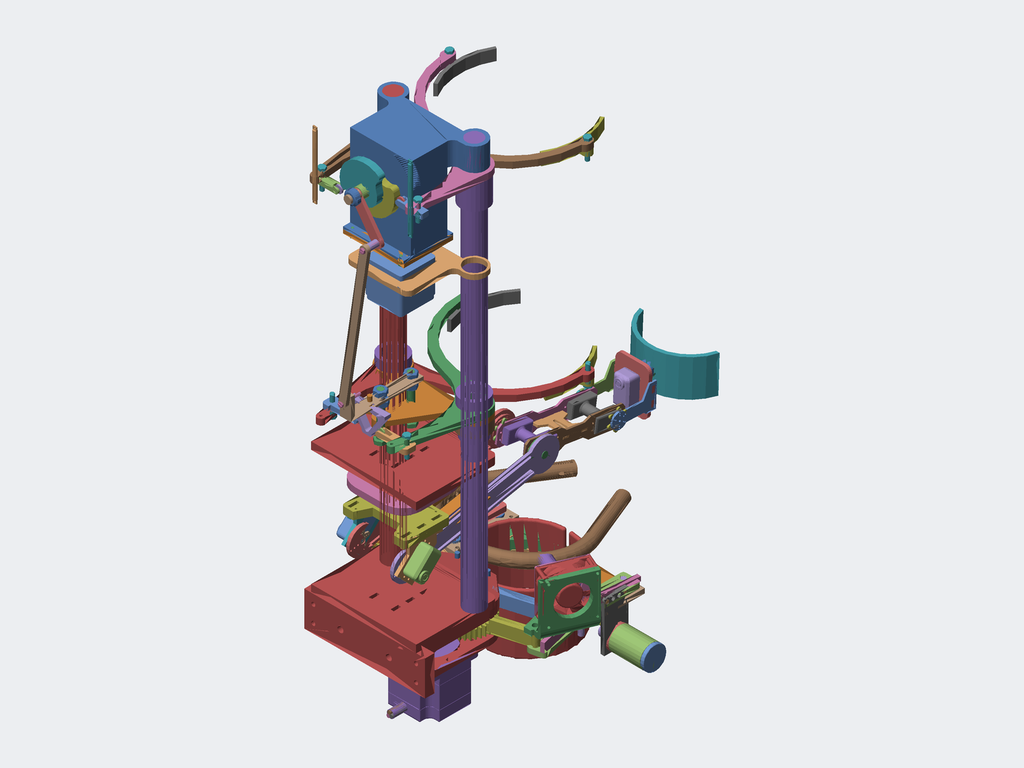Assembly | SolidWorks | 153 different items | 184 placed
Parts list (item | name | quantity | size | volume | features):
1 | (subassembly) | x1 | 346.952 x 128.874 x 340.963 mm | 1244535 mm3 | -
2 | - | x2 | 48 x 48 x 18 mm | 12158 mm3 | features Extrusion 1
3 | - | x1 | 42.805 x 27 x 33.95 mm | 11771 mm3 | features BaseBody 1
4 | - | x1 | 73.253 x 17.318 x 324 mm | 124814 mm3 | features BaseBody 1
5 | - | x1 | 225.335 x 227.919 x 57.4 mm | 931418 mm3 | features Cut 5, HoleWzd 5, ICE 3, Extrusion 1, Fillet 1
6 | - | x1 | 53.735 x 9.545 x 80 mm | 17956 mm3 | features BaseBody 1
7 | - | x1 | 20 x 23 x 32 mm | 12308 mm3 | features BaseBody 1
8 | - | x1 | 60 x 84 x 72 mm | 236948 mm3 | features ICE 5, Fillet 2, Chamfer 1, Extrusion 1
9 | - | x1 | 172 x 114 x 8 mm | 50080 mm3 | features Extrusion 1
10 | - | x1 | 40 x 24 x 32 mm | 2333 mm3 | features BaseBody 1
11 | - | x1 | 45 x 65 x 20 mm | 41025 mm3 | features BaseBody 1
12 | - | x1 | 40.811 x 30 x 4 mm | 1334 mm3 | features BaseBody 1
13 | - | x1 | 216 x 275.5 x 10 mm | 64163 mm3 | features Extrusion 1
14 | - | x1 | 200 x 37.759 x 140 mm | 122488 mm3 | features BaseBody 1
15 | - | x1 | 75.848 x 62.021 x 10 mm | 29978 mm3 | features Extrusion 1, ICE 1
16 | - | x1 | 75.848 x 62.021 x 10 mm | 30038 mm3 | features Extrusion 1, ICE 1
17 | - | x1 | 19.1 x 9.5 x 9.534 mm | 562.61 mm3 | features Extrusion 1, Fillet 1, ICE 1
18 | - | x1 | 19.1 x 9.5 x 9.534 mm | 562.61 mm3 | features Extrusion 1, Fillet 1, ICE 1
19 | - | x1 | 60 x 40 x 10 mm | 8175 mm3 | features Extrusion 1, ICE 1
20 | - | x1 | 23 x 23 x 4.6 mm | 774.952 mm3 | features Extrusion 1, ICE 1
21 | - | x1 | 39.607 x 26.395 x 3 mm | 406.832 mm3 | features BaseBody 1
22 | - | x1 | 31 x 75 x 3 mm | 697.725 mm3 | features BaseBody 1
23 | - | x1 | 102.526 x 43 x 3 mm | 1128 mm3 | features BaseBody 1
24 | - | x1 | 216 x 259.5 x 10 mm | 61129 mm3 | features Extrusion 1
25 | - | x1 | 30 x 13 x 10 mm | 1236 mm3 | features BaseBody 1
26 | - | x1 | 24.142 x 77.176 x 18 mm | 8760 mm3 | features BaseBody 1
27 | - | x1 | 20 x 20 x 20 mm | 5278 mm3 | features Extrusion 1
28 | - | x1 | 14.483 x 32 x 22.5 mm | 7805 mm3 | features BaseBody 1
29 | - | x1 | 28.933 x 49.206 x 26 mm | 4873 mm3 | features BaseBody 1
30 | - | x1 | 19.494 x 47.938 x 13 mm | 3166 mm3 | features BaseBody 1
31 | - | x1 | 29 x 12 x 12 mm | 1793 mm3 | features BaseBody 1
32 | - | x1 | 25.14 x 25.14 x 72 mm | 10941 mm3 | features BaseBody 1
33 | - | x1 | 8 x 14 x 80 mm | 2633 mm3 | features BaseBody 1
34 | - | x1 | 20 x 40 x 41 mm | 9841 mm3 | features BaseBody 1
35 | - | x1 | 44 x 12 x 8 mm | 3492 mm3 | features Extrusion 1, Fillet 1, ICE 1
36 | - | x1 | 42 x 13 x 13 mm | 2716 mm3 | features Chamfer 2, ICE 2, Revolution 1
37 | - | x1 | 114 x 17 x 17 mm | 14497 mm3 | features ICE 2, Revolution 1
38 | - | x1 | 18 x 18 x 10 mm | 1338 mm3 | features Extrusion 1
39 | - | x1 | 120 x 18 x 36 mm | 15012 mm3 | features ICE 5, Extrusion 1
40 | - | x1 | 12 x 106 x 27.4 mm | 23043 mm3 | features ICE 2, Extrusion 1, Fillet 1
41 | - | x1 | 12 x 106 x 27.4 mm | 23043 mm3 | features ICE 2, Extrusion 1, Fillet 1
42 | - | x1 | 77.185 x 16 x 5 mm | 5210 mm3 | features Extrusion 1
43 | - | x1 | 10 x 10 x 15.5 mm | 1023 mm3 | features Extrusion 1
44 | - | x1 | 252 x 12 x 6 mm | 17808 mm3 | features Extrusion 1
45 | - | x1 | 222.738 x 50.026 x 174 mm | 466487 mm3 | features BaseBody 1
46 | - | x1 | 44 x 12 x 8 mm | 3492 mm3 | features Extrusion 1, Fillet 1, ICE 1
47 | - | x1 | 60 x 84 x 72 mm | 237017 mm3 | features ICE 4, Fillet 2, Chamfer 1, Extrusion 1
48 | - | x1 | 216 x 263.5 x 15 mm | 92831 mm3 | features Extrusion 1
49 | - | x1 | 216 x 259.5 x 15 mm | 91694 mm3 | features Extrusion 1
50 | - | x1 | 2.5 x 53.856 x 24.571 mm | 1339 mm3 | features ICE 4, MoveCopyBody 1, Stock 1
51 | - | x1 | 2.5 x 53.856 x 24.571 mm | 1339 mm3 | features ICE 4, MoveCopyBody 1, Stock 1
52 | - | x1 | 90 x 15 x 10 mm | 13500 mm3 | features BaseBody 1
53 | - | x1 | 23.5 x 40.616 x 37 mm | 6167 mm3 | features BaseBody 1
54 | - | x1 | 105.6 x 75 x 12 mm | 72869 mm3 | features Extrusion 1
55 | - | x1 | 70 x 36.517 x 5 mm | 8161 mm3 | features Fillet 3, Extrusion 1
56 | - | x1 | 70 x 36.517 x 5 mm | 8161 mm3 | features Fillet 3, Extrusion 1
57 | - | x1 | 75.329 x 67.7 x 5 mm | 9212 mm3 | features Extrusion 1
58 | - | x1 | 75.329 x 67.7 x 5 mm | 9212 mm3 | features Extrusion 1
59 | - | x1 | 42.5 x 72.6 x 3 mm | 4588 mm3 | features Extrusion 1
60 | - | x1 | 33.41 x 29.789 x 5.85 mm | 1360 mm3 | features ICE 4, Extrusion 1, Fillet 1
61 | - | x1 | 33.41 x 29.789 x 5.85 mm | 1360 mm3 | features ICE 4, Extrusion 1, Fillet 1
62 | - | x1 | 33.41 x 29.789 x 5.85 mm | 1360 mm3 | features ICE 4, Extrusion 1, Fillet 1
63 | - | x1 | 33.41 x 29.789 x 5.85 mm | 1360 mm3 | features ICE 4, Extrusion 1, Fillet 1
64 | - | x1 | 33.41 x 29.789 x 5.85 mm | 1360 mm3 | features ICE 4, Extrusion 1, Fillet 1
65 | - | x1 | 33.41 x 29.789 x 5.85 mm | 1360 mm3 | features ICE 4, Extrusion 1, Fillet 1
66 | - | x1 | 33.41 x 29.789 x 5.85 mm | 1360 mm3 | features ICE 4, Extrusion 1, Fillet 1
67 | - | x1 | 171 x 118.5 x 140 mm | 515598 mm3 | features ICE 7, RevCut 2, Extrusion 1
68 | - | x1 | 82 x 100 x 14 mm | 49472 mm3 | features ICE 5, Extrusion 1
69 | - | x1 | 45.38 x 20.336 x 45.38 mm | 6966 mm3 | features BaseBody 1
70 | - | x1 | 65.7 x 75 x 5 mm | 16997 mm3 | features Extrusion 1, Fillet 1, ICE 1
71 | - | x1 | 50 x 20 x 50 mm | 8321 mm3 | features BaseBody 1
72 | - | x1 | - | - | features ICE 2, CirPattern 1, Extrusion 1, Helix 1, RefAxis 1, SweepCut 1
73 | - | x1 | 279.515 x 6.264 x 50 mm | 42669 mm3 | features ICE 3, Extrusion 1
74 | - | x1 | 279.515 x 6.264 x 50 mm | 42669 mm3 | features ICE 3, Extrusion 1
75 | - | x1 | 79 x 77.9 x 5 mm | 23665 mm3 | features Extrusion 1, ICE 1
76 | - | x1 | 77.052 x 77.02 x 12.051 mm | 23159 mm3 | features RefAxis 2, Revolution 2, BlendCut 1, CirPattern 1, ICE 1
77 | - | x1 | 671 x 37 x 37 mm | 528385 mm3 | features Revolution 1
78 | - | x1 | 671 x 44 x 44 mm | 560064 mm3 | features Revolution 1
79 | - | x1 | 17.234 x 17.234 x 54 mm | 6790 mm3 | features ICE 6, Chamfer 1, CirPattern 1, Extrusion 1, Helix 1, RefAxis 1, SweepCut 1
80 | - | x1 | 164.86 x 31.5 x 3 mm | 8343 mm3 | features Extrusion 1
81 | - | x1 | 54 x 20 x 8 mm | 4696 mm3 | features Fillet 2, ICE 2, Extrusion 1
82 | - | x1 | 164.86 x 31.5 x 3 mm | 8343 mm3 | features Extrusion 1
83 | - | x1 | 50 x 49.3 x 3 mm | 5034 mm3 | features Extrusion 1
84 | - | x1 | 40 x 15 x 40 mm | 6357 mm3 | features ICE 5, Extrusion 1
85 | - | x1 | 40 x 13.2 x 40 mm | 4095 mm3 | features ICE 5, Extrusion 1
86 | - | x1 | 41.5 x 21.5 x 55 mm | 30038 mm3 | features ICE 6, Chamfer 1, Extrusion 1, Fillet 1
87 | - | x1 | 41.5 x 21.5 x 55 mm | 30038 mm3 | features ICE 6, Chamfer 1, Extrusion 1, Fillet 1
88 | - | x1 | 29.446 x 29.325 x 13.992 mm | 4731 mm3 | features RefAxis 2, BlendCut 1, CirPattern 1, Revolution 1
89 | - | x1 | 50.144 x 42.117 x 46.062 mm | 27040 mm3 | features ICE 3, Fillet 2, Chamfer 1, Cut 1, Extrusion 1
90 | - | x1 | 50.144 x 42.117 x 46.062 mm | 27040 mm3 | features ICE 3, Fillet 2, Chamfer 1, Cut 1, Extrusion 1
91 | - | x1 | 50.144 x 42.117 x 46.062 mm | 27040 mm3 | features ICE 3, Fillet 2, Chamfer 1, Cut 1, Extrusion 1
92 | - | x1 | 54 x 20 x 8 mm | 4696 mm3 | features Fillet 2, ICE 2, Extrusion 1
93 | - | x2 | 174 x 136 x 12 mm | 259651 mm3 | features Extrusion 1, Fillet 1
94 | - | x1 | 110 x 110 x 25 mm | 105460 mm3 | features Fillet 2, ICE 2, Extrusion 1
95 | - | x1 | 50 x 50 x 36 mm | 14585 mm3 | features ICE 4, Extrusion 1
96 | - | x2 | 80 x 139.91 x 27.4 mm | 82359 mm3 | features ICE 3, Extrusion 1, Fillet 1
97 | - | x1 | 27.226 x 27.226 x 15 mm | 4643 mm3 | features Extrusion 1
98 | - | x1 | 6 x 6 x 110 mm | 2900 mm3 | features ICE 4, Extrusion 1
99 | - | x1 | 6 x 6 x 110 mm | 2900 mm3 | features ICE 4, Extrusion 1
100 | - | x2 | 20 x 20 x 10 mm | 2867 mm3 | features HoleWzd 2, Cut 1, Extrusion 1
101 | - | x4 | 3 x 3 x 13 mm | 89.797 mm3 | features Chamfer 1, Extrusion 1
102 | - | x4 | 12 x 12 x 46 mm | 2501 mm3 | features ICE 3, Extrusion 1
103 | - | x1 | 216 x 275.5 x 10 mm | 60864 mm3 | features Extrusion 1
104 | - | x2 | 31.948 x 20.133 x 14.168 mm | 1802 mm3 | features Cut 7, ICE 5, Extrusion 1, HoleWzd 1
105 | - | x2 | 111.649 x 70.016 x 8 mm | 27509 mm3 | features HoleWzd 3, ICE 3, Cut 1, Extrusion 1
106 | - | x2 | 6 x 19 x 6.001 mm | 500.74 mm3 | features Cut 3, Extrusion 1, HoleWzd 1
107 | - | x4 | 20 x 20 x 11 mm | 1797 mm3 | features Chamfer 1, Extrusion 1, ICE 1
108 | - | x2 | 5 x 5 x 15 mm | 142.965 mm3 | features ICE 2, Cut 1, Extrusion 1
109 | - | x2 | 5 x 5 x 19.999 mm | 180.305 mm3 | features ICE 2, Cut 1, Extrusion 1
110 | - | x1 | 176.98 x 108.741 x 8 mm | 42748 mm3 | features Cut 1, Extrusion 1
111 | - | x1 | 176.98 x 108.741 x 8 mm | 42748 mm3 | features Cut 1, Extrusion 1
112 | - | x1 | 166.528 x 92.061 x 15 mm | 14282 mm3 | features HoleWzd 2, Cut 1, Extrusion 1
113 | - | x1 | 166.528 x 92.061 x 15 mm | 14282 mm3 | features Cut 2, Extrusion 1, HoleWzd 1
114 | - | x1 | 216 x 275.5 x 10 mm | 60864 mm3 | features Extrusion 1
115 | - | x4 | 6 x 6 x 12 mm | 334.841 mm3 | features Chamfer 2, Extrusion 1
116 | - | x1 | 39.504 x 80 x 6.135 mm | 17187 mm3 | features Cut 2, HoleWzd 2, Extrusion 1
117 | - | x1 | 39.504 x 80 x 6.135 mm | 17187 mm3 | features Cut 2, HoleWzd 2, Extrusion 1
118 | - | x1 | 114.513 x 126.581 x 23 mm | 34516 mm3 | features Cut 4, HoleWzd 2, Extrusion 1, ICE 1
119 | - | x1 | 84.083 x 77.703 x 6 mm | 11123 mm3 | features Extrusion 1, ICE 1
120 | - | x1 | 88.743 x 86.001 x 87 mm | 61033 mm3 | features Cut 2, ICE 2, RefAxis 2, EdgeFlange 1, FlatPattern 1, SMBaseFlange 1, SheetMetal 1
121 | - | x2 | 70 x 70 x 25 mm | 39371 mm3 | features ICE 10, Fillet 8, CirPattern 2, MirrorPattern 2, CombineBodies 1, Extrusion 1, Helix 1, RevCut 1, Sweep 1
122 | - | x1 | 86.705 x 77.475 x 87.001 mm | 59436 mm3 | features Cut 1, EdgeFlange 1, FlatPattern 1, ICE 1, SMBaseFlange 1, SheetMetal 1
123 | - | x2 | 238.083 x 103.353 x 20 mm | 30963 mm3 | features RevCut 2, CirPattern 1, Cut 1, RefAxis 1, Sweep 1
124 | - | x2 | 50 x 50 x 56.352 mm | 10137 mm3 | features ICE 2, Blend 1, Cut 1, Extrusion 1, RefAxis 1, RevCut 1, SweepCut 1
125 | - | x1 | 182 x 122.5 x 22 mm | 68800 mm3 | features Extrusion 1, ICE 1
126 | - | x2 | 70 x 70 x 2 mm | 5744 mm3 | features Cut 2, FlatPattern 1, SMBaseFlange 1, SheetMetal 1
127 | - | x4 | 14 x 14 x 65.4 mm | 3691 mm3 | features ICE 2, Cut 1, Extrusion 1
128 | - | x1 | 114.513 x 126.581 x 23 mm | 34944 mm3 | features Cut 5, ICE 5, RevCut 3, HoleWzd 2, Extrusion 1
129 | - | x1 | 84.083 x 77.703 x 6 mm | 11123 mm3 | features Extrusion 1, ICE 1
130 | - | x2 | 139.296 x 94.506 x 100 mm | 127694 mm3 | features ICE 2, Extrusion 1, Fillet 1
131 | - | x1 | 24.068 x 19.259 x 24 mm | 2234 mm3 | features ICE 5, Fillet 2, Chamfer 1, Extrusion 1
132 | - | x1 | 12 x 12 x 2 mm | 201.062 mm3 | features Extrusion 1
133 | - | x1 | 12 x 12 x 2 mm | 201.062 mm3 | features Extrusion 1
134 | - | x1 | 12 x 12 x 2 mm | 201.062 mm3 | features Extrusion 1
135 | - | x1 | 12 x 12 x 2 mm | 201.062 mm3 | features Extrusion 1
136 | - | x2 | 44 x 44 x 63 mm | 26578 mm3 | features Extrusion 1, ICE 1
137 | - | x1 | 51.978 x 130.553 x 60 mm | 56854 mm3 | features Extrusion 1, ICE 1
138 | - | x1 | 35.397 x 105 x 18 mm | 11366 mm3 | features Extrusion 1, ICE 1
139 | - | x1 | 35.397 x 105 x 18 mm | 11366 mm3 | features Extrusion 1, ICE 1
140 | - | x1 | 35.397 x 105 x 18 mm | 11366 mm3 | features Extrusion 1, ICE 1
141 | - | x1 | 35.397 x 105 x 18 mm | 11366 mm3 | features Extrusion 1, ICE 1
142 | - | x1 | 85 x 105 x 109 mm | 475306 mm3 | features ICE 14, Fillet 8, Chamfer 3, CirPattern 2, Extrusion 1, MirrorPattern 1
143 | - | x1 | 50 x 43 x 48 mm | 49165 mm3 | features BaseBody 1
144 | - | x1 | 15 x 43.5 x 27 mm | 2257 mm3 | features BaseBody 1
145 | - | x1 | 55 x 55 x 44 mm | 106147 mm3 | features BaseBody 1
146 | - | x2 | 38 x 42.771 x 84 mm | 72893 mm3 | features Chamfer 4, Revolution 4, ICE 3, MirrorPattern 1, RefAxis 1
147 | - | x1 | 42.5 x 72.6 x 3 mm | 4588 mm3 | features Extrusion 1
148 | cross recessed hex bolts indentation gb | x1 | - | - | -
149 | hex bolts split pin hole-fine pitch-ab gb | x1 | - | - | -
150 | hex bolts with slot on head grade ab gb | x1 | - | - | -
151 | hex bolts with split pin hole-grade ab gb | x1 | - | - | -
152 | hex nuts 1-fine pitch-grades ab gb | x1 | - | - | -
153 | round nuts gb | x1 | - | - | -
Mates (type | each side: item.copy, entity, surface, feature):
Concentric | 67.1 face cylinder Boss-Extrude 1 | 78.1 face cylinder Revolve 1 | 2 times
Coincident | 67.1 edge | 78.1 edge
Concentric | 67.1 face cylinder Boss-Extrude 1 | 77.1 face cylinder Revolve 1
Coincident | 67.1 edge | 77.1 edge
Concentric | 77.1 face cylinder Revolve 1 | 13.1 face cylinder Boss-Extrude 1
Coincident | 77.1 face plane Revolve 1 | 13.1 face plane Boss-Extrude 1
Concentric | 78.1 face cylinder Revolve 1 | 24.1 face cylinder Boss-Extrude 1
Coincident | 78.1 face plane Revolve 1 | 24.1 face plane Boss-Extrude 1
Concentric | 24.1 face cylinder Boss-Extrude 1 | 140.1 face cylinder Boss-Extrude 5
Coincident | 24.1 face plane Boss-Extrude 1 | 140.1 face plane Boss-Extrude 5
Concentric | 13.1 face cylinder Boss-Extrude 1 | 141.1 face cylinder Boss-Extrude 5
Coincident | 13.1 face plane Boss-Extrude 1 | 141.1 face plane Boss-Extrude 5
Concentric | 24.1 face cylinder Boss-Extrude 1 | 98.1 face cylinder Boss-Extrude 1
Concentric | 13.1 face cylinder Boss-Extrude 1 | 99.1 face cylinder Boss-Extrude 1
Concentric | 24.1 face cylinder Boss-Extrude 1 | 35.1 face cylinder Boss-Extrude 1
Coincident | 24.1 face plane Boss-Extrude 1 | 35.1 face plane Boss-Extrude 1
Concentric | 35.1 face cylinder Boss-Extrude 2 | 132.1 face cylinder Boss-Extrude 1
DistanceDim | 132.1 face plane Boss-Extrude 1 | 35.1 face plane Boss-Extrude 1
Concentric | 13.1 face cylinder Boss-Extrude 1 | 46.1 face cylinder Boss-Extrude 1
Coincident | 13.1 face plane Boss-Extrude 1 | 46.1 face plane Boss-Extrude 1
Concentric | 46.1 face cylinder Boss-Extrude 2 | 133.1 face cylinder Boss-Extrude 1
DistanceDim | 133.1 face plane Boss-Extrude 1 | 46.1 face plane Boss-Extrude 1
Concentric | 67.1 face cylinder Cut-Revolve 3 | 37.1 face cylinder Revolve 1
Concentric | 37.1 face cylinder Revolve 1 | 72.1 face cylinder Cut-Extrude 1
Coincident | 67.1 face plane Boss-Extrude 7 | 72.1 face plane 0.80000 模数 , 78.1710mm P.D.
Concentric | 67.1 face cylinder Cut-Revolve 4 | 79.1 face cylinder Boss-Extrude 2
Coincident | 67.1 face plane Boss-Extrude 7 | 79.1 face plane Boss-Extrude 3
Concentric | 79.1 face cylinder Boss-Extrude 2 | 76.1 face cylinder 1.5 模数    , 76.5000mm P.D.
Coincident | 67.1 face plane Boss-Extrude 7 | 76.1 face plane Hub-Revolve1
Concentric | 68.1 face cylinder Cut-Extrude 9 | 20.1 face cylinder Boss-Extrude 2
Coincident | 68.1 face plane Boss-Extrude 3 | 20.1 edge
Concentric | 20.1 face cylinder Boss-Extrude 2 | 27.1 face cylinder Boss-Extrude 1
Coincident | 20.1 face plane Boss-Extrude 1 | 27.1 face plane Boss-Extrude 1
Concentric | 68.1 face cylinder Cut-Extrude 8 | 36.1 face cylinder Revolve 2
Coincident | 20.1 face plane Boss-Extrude 1 | 36.1 face plane Revolve 2
Concentric | 36.1 face cylinder Revolve 2 | 88.1 face cylinder 1.5 模数    , 25.5000mm P.D.
DistanceDim | 88.1 face plane 1.5 模数    , 25.5000mm P.D. | 36.1 face plane Revolve 2
Coincident | 67.1 face plane Boss-Extrude 1 | 37.1 face plane Revolve 1
Concentric | 37.1 face cylinder Revolve 1 | 15.1 face cylinder Boss-Extrude 1
Concentric | 37.1 face cylinder Revolve 1 | 16.1 face cylinder Boss-Extrude 1
ProfileCenter | 67.1 face plane Boss-Extrude 7 | 68.1 face plane Boss-Extrude 1
Concentric | 27.1 face cylinder Boss-Extrude 1 | 8.1 face cylinder Boss-Extrude 2
Coincident | 27.1 face plane Boss-Extrude 1 | 8.1 face plane Boss-Extrude 1
Concentric | 77.1 face cylinder Revolve 1 | 9.1 face cylinder Boss-Extrude 1
Concentric | 78.1 face cylinder Revolve 1 | 9.1 face cylinder Boss-Extrude 1
DistanceDim | 9.1 face plane Boss-Extrude 1 | 68.1 face plane Boss-Extrude 1
Parallel | 67.1 face plane Boss-Extrude 1 | 15.1 face plane Boss-Extrude 2 | 2 times
CamTangent | 15.1 face surface:4009 Boss-Extrude 2 | 132.1 face cylinder Boss-Extrude 1
Concentric | 37.1 face cylinder Revolve 1 | 38.1 face cylinder Boss-Extrude 1
Coincident | 16.1 face plane Boss-Extrude 2 | 38.1 face plane Boss-Extrude 1
Concentric | 37.1 face cylinder Revolve 1 | 42.1 face cylinder Boss-Extrude 1
Concentric | 42.1 face cylinder Boss-Extrude 1 | 43.1 face cylinder Boss-Extrude 1
Coincident | 42.1 face plane Boss-Extrude 1 | 43.1 face plane Boss-Extrude 1
Concentric | 43.1 face cylinder Boss-Extrude 1 | 44.1 face cylinder Boss-Extrude 1
Coincident | 43.1 face plane Boss-Extrude 1 | 44.1 face plane Boss-Extrude 1
Parallel | 37.1 face plane Cut-Extrude 1 | 38.1 face plane Boss-Extrude 1
Parallel | 38.1 face plane Boss-Extrude 1 | 42.1 face plane Boss-Extrude 1
Parallel | 37.1 face plane Cut-Extrude 1 | 15.1 face plane Boss-Extrude 2 | 2 times
Parallel | 37.1 face plane Cut-Extrude 1 | 16.1 face plane Boss-Extrude 2
Coincident | 15.1 face plane Boss-Extrude 2 | 16.1 face plane Boss-Extrude 2
CamTangent | 16.1 face surface:4009 Boss-Extrude 2 | 133.1 face cylinder Boss-Extrude 1
Concentric | 78.1 face cylinder Revolve 1 | 125.1 face cylinder Boss-Extrude 1
Concentric | 77.1 face cylinder Revolve 1 | 125.1 face cylinder Boss-Extrude 1
Parallel | 9.1 face plane Boss-Extrude 1 | 125.1 face plane Boss-Extrude 1
Concentric | 125.1 face cylinder Boss-Extrude 1 | 114.1 face cylinder Boss-Extrude 3
Coincident | 125.1 face plane Boss-Extrude 1 | 114.1 face plane Boss-Extrude 3
Concentric | 125.1 face cylinder Boss-Extrude 1 | 103.1 face cylinder Boss-Extrude 3
Coincident | 125.1 face plane Boss-Extrude 1 | 103.1 face plane Boss-Extrude 3
Concentric | 78.1 face cylinder Revolve 1 | 136.1 face cylinder Boss-Extrude 1
Coincident | 103.1 face plane Boss-Extrude 3 | 136.1 face plane Boss-Extrude 1
Coincident | 125.1 face plane Boss-Extrude 1 | 2.1 face plane Boss-Extrude 1
Concentric | 78.1 face cylinder Revolve 1 | 2.1 face cylinder Boss-Extrude 1
Concentric | 77.1 face cylinder Revolve 1 | 136.2 face cylinder Boss-Extrude 1
Coincident | 125.1 face plane Boss-Extrude 1 | 136.2 face plane Boss-Extrude 1
Concentric | 77.1 face cylinder Revolve 1 | 2.2 face cylinder Boss-Extrude 1
Coincident | 114.1 face plane Boss-Extrude 3 | 2.2 face plane Boss-Extrude 1
Concentric | 103.1 face cylinder Boss-Extrude 3 | 138.1 face cylinder Boss-Extrude 5
Coincident | 103.1 face plane Boss-Extrude 3 | 138.1 face plane Boss-Extrude 5
Concentric | 114.1 face cylinder Boss-Extrude 3 | 139.1 face cylinder Boss-Extrude 5
Coincident | 114.1 face plane Boss-Extrude 3 | 139.1 face plane Boss-Extrude 5
Concentric | 103.1 face cylinder Boss-Extrude 3 | 81.1 face cylinder Cut-Extrude 1
Coincident | 103.1 face plane Boss-Extrude 3 | 81.1 face plane Boss-Extrude 1
Concentric | 81.1 face cylinder Boss-Extrude 2 | 134.1 face cylinder Boss-Extrude 1
DistanceDim | 81.1 face plane Boss-Extrude 1 | 134.1 face plane Boss-Extrude 1
Concentric | 114.1 face cylinder Boss-Extrude 3 | 92.1 face cylinder Cut-Extrude 1
Concentric | 92.1 face cylinder Boss-Extrude 2 | 135.1 face cylinder Boss-Extrude 1
DistanceDim | 92.1 face plane Boss-Extrude 1 | 135.1 face plane Boss-Extrude 1
Coincident | 114.1 face plane Boss-Extrude 3 | 92.1 face plane Boss-Extrude 1
Coincident | 19.1 face plane Boss-Extrude 1 | 39.1 face plane Boss-Extrude 1
Concentric | 19.1 face cylinder Cut-Extrude 1 | 39.1 face cylinder Cut-Extrude 3
Parallel | 19.1 face plane Boss-Extrude 1 | 39.1 face plane Boss-Extrude 3
Tangent | 134.1 face cylinder Boss-Extrude 1 | 19.1 face plane Boss-Extrude 1
Tangent | 135.1 face cylinder Boss-Extrude 1 | 19.1 face plane Boss-Extrude 1
Concentric | 44.1 face cylinder Boss-Extrude 1 | 39.1 face cylinder Cut-Extrude 4
Parallel | 37.1 face plane Cut-Extrude 1 | 42.1 face plane Boss-Extrude 1
Coincident | 38.1 face plane Boss-Extrude 1 | 42.1 face plane Boss-Extrude 1
Coincident | 44.1 face plane Boss-Extrude 1 | 39.1 face plane Boss-Extrude 3
Parallel | 125.1 face cylinder Boss-Extrude 1 | 39.1 face cylinder Cut-Extrude 1 | 2 times
Concentric | 125.1 face cylinder Boss-Extrude 1 | 39.1 face cylinder Cut-Extrude 1 | 2 times
Concentric | 78.1 face cylinder Revolve 1 | 93.1 face cylinder Boss-Extrude 1
Concentric | 77.1 face cylinder Revolve 1 | 93.1 face cylinder Boss-Extrude 1
Coincident | 93.1 face plane Boss-Extrude 1 | 56.1 face plane Boss-Extrude 1 | 3 times
Coincident | 93.1 face plane Boss-Extrude 1 | 55.1 face plane Boss-Extrude 1 | 3 times
Coincident | 56.1 face plane Boss-Extrude 1 | 94.1 face plane Boss-Extrude 1 | 3 times
Concentric | 94.1 face cylinder Cut-Extrude 1 | 95.1 face cylinder Boss-Extrude 3
Coincident | 94.1 face plane Boss-Extrude 2 | 95.1 face plane Boss-Extrude 2
Concentric | 95.1 face cylinder Boss-Extrude 5 | 54.1 face cylinder Boss-Extrude 1
Coincident | 95.1 face plane Boss-Extrude 4 | 54.1 face plane Boss-Extrude 1
Coincident | 54.1 face plane Boss-Extrude 1 | 57.1 face plane Boss-Extrude 1 | 3 times
Coincident | 54.1 face plane Boss-Extrude 1 | 58.1 face plane Boss-Extrude 1 | 3 times
Coincident | 57.1 face plane Boss-Extrude 1 | 89.1 face plane Boss-Extrude 1 | 3 times
Coincident | 58.1 face plane Boss-Extrude 1 | 90.1 face plane Boss-Extrude 1 | 3 times
Coincident | 89.1 face plane Boss-Extrude 1 | 60.1 face plane Boss-Extrude 1
Coincident | 90.1 face plane Boss-Extrude 1 | 61.1 face plane Boss-Extrude 1
Coincident | 73.1 face plane Boss-Extrude 1 | 60.1 face plane Boss-Extrude 1
Coincident | 74.1 face plane Boss-Extrude 1 | 61.1 face plane Boss-Extrude 1
Concentric | 90.1 face cylinder Boss-Extrude 4 | 61.1 face cylinder Cut-Extrude 1
Concentric | 89.1 face cylinder Boss-Extrude 4 | 60.1 face cylinder Cut-Extrude 1
Coincident | 73.1 face plane Boss-Extrude 1 | 74.1 face plane Boss-Extrude 1
Concentric | 74.1 face cylinder Boss-Extrude 1 | 84.1 face cylinder Boss-Extrude 2
Coincident | 74.1 face plane Boss-Extrude 1 | 84.1 face plane Boss-Extrude 1
Concentric | 84.1 face cylinder Boss-Extrude 3 | 62.1 face cylinder Cut-Extrude 1
Coincident | 84.1 face plane Boss-Extrude 1 | 62.1 face plane Boss-Extrude 1
Coincident | 62.1 face plane Boss-Extrude 1 | 86.1 face plane Boss-Extrude 3
Concentric | 62.1 face cylinder Boss-Extrude 2 | 86.1 face cylinder Cut-Extrude 3
Coincident | 86.1 face plane Boss-Extrude 3 | 80.1 face plane Boss-Extrude 3 | 2 times
DistanceDim | 86.1 face plane Boss-Extrude 3 | 80.1 face plane Boss-Extrude 3
Coincident | 86.1 face plane Boss-Extrude 1 | 82.1 face plane Boss-Extrude 3 | 2 times
DistanceDim | 82.1 face plane Boss-Extrude 3 | 86.1 face plane Boss-Extrude 1
Coincident | 80.1 face plane Boss-Extrude 3 | 87.1 face plane Boss-Extrude 3 | 2 times
DistanceDim | 87.1 face plane Boss-Extrude 3 | 80.1 face plane Boss-Extrude 3
Concentric | 87.1 face cylinder Cut-Extrude 3 | 64.1 face cylinder Boss-Extrude 2
Coincident | 87.1 face plane Boss-Extrude 3 | 64.1 face plane Boss-Extrude 1
Concentric | 87.1 face cylinder Cut-Extrude 1 | 65.1 face cylinder Boss-Extrude 2
Coincident | 87.1 face plane Boss-Extrude 1 | 65.1 face plane Boss-Extrude 1
Concentric | 64.1 face cylinder Cut-Extrude 1 | 147.1 face cylinder Boss-Extrude 1
Coincident | 64.1 face plane Boss-Extrude 1 | 147.1 face plane Boss-Extrude 1
Concentric | 65.1 face cylinder Cut-Extrude 1 | 59.1 face cylinder Boss-Extrude 1
Coincident | 65.1 face plane Boss-Extrude 1 | 59.1 face plane Boss-Extrude 1
Coincident | 80.1 face plane Boss-Extrude 3 | 83.1 face plane Boss-Extrude 1 | 3 times
Coincident | 147.1 face plane Boss-Extrude 1 | 70.1 face plane Boss-Extrude 1 | 2 times
DistanceDim | 70.1 face plane Boss-Extrude 1 | 59.1 face plane Boss-Extrude 1
Coincident | 59.1 face plane Boss-Extrude 1 | 70.1 face plane Boss-Extrude 1
Coincident | 70.1 face plane Cut-Extrude 1 | 91.1 face plane Boss-Extrude 1 | 2 times
Coincident | 70.1 face plane Boss-Extrude 1 | 91.1 face plane Boss-Extrude 1
Concentric | 91.1 face cylinder Boss-Extrude 4 | 66.1 face cylinder Cut-Extrude 1
Coincident | 91.1 face plane Boss-Extrude 1 | 66.1 face plane Boss-Extrude 1
Concentric | 74.1 face cylinder Boss-Extrude 1 | 61.1 face cylinder Boss-Extrude 2
Coincident | 74.1 face plane Cut-Extrude 3 | 75.1 face plane Boss-Extrude 1 | 2 times
Coincident | 74.1 face plane Boss-Extrude 1 | 75.1 face plane Boss-Extrude 1
Concentric | 66.1 face cylinder Cut-Extrude 1 | 131.1 face cylinder Boss-Extrude 6
Coincident | 66.1 face plane Boss-Extrude 2 | 131.1 face plane Boss-Extrude 4
Concentric | 131.1 face cylinder Boss-Extrude 2 | 17.1 face cylinder Boss-Extrude 2
Coincident | 131.1 face plane Boss-Extrude 1 | 17.1 face plane Boss-Extrude 1
Parallel | 131.1 face plane Boss-Extrude 1 | 17.1 face plane Boss-Extrude 1
Concentric | 131.1 face cylinder Boss-Extrude 2 | 18.1 face cylinder Boss-Extrude 2
Coincident | 131.1 face plane Boss-Extrude 1 | 18.1 face plane Boss-Extrude 1
Parallel | 17.1 face plane Boss-Extrude 1 | 18.1 face plane Boss-Extrude 1
Concentric | 5.1 face cylinder Cut-Extrude 2 | 142.1 face cylinder Boss-Extrude 3
Coincident | 5.1 face plane Boss-Extrude 1 | 142.1 face plane Boss-Extrude 2
Concentric | 5.1 face cylinder Cut-Extrude 4 | 96.1 face cylinder Cut-Extrude 2
Coincident | 5.1 face plane Boss-Extrude 3 | 96.1 face plane Boss-Extrude 2
Concentric | 5.1 face cylinder Cut-Extrude 4 | 96.2 face cylinder Cut-Extrude 2
Coincident | 5.1 face plane Boss-Extrude 3 | 96.2 face plane Boss-Extrude 2
Parallel | 5.1 face plane Boss-Extrude 4 | 142.1 face plane Boss-Extrude 1
Concentric | 142.1 face cylinder Boss-Extrude 3 | 97.1 face cylinder Boss-Extrude 1
Coincident | 142.1 face plane Boss-Extrude 3 | 97.1 face plane Boss-Extrude 1
Concentric | 5.1 face cylinder M6 Tapped Hole 2 | 40.1 face cylinder Cut-Extrude 1
Coincident | 5.1 face plane Boss-Extrude 3 | 40.1 face plane Boss-Extrude 1
Concentric | 5.1 face cylinder M6 Tapped Hole 2 | 41.1 face cylinder Cut-Extrude 1
Coincident | 5.1 face plane Boss-Extrude 3 | 41.1 face plane Boss-Extrude 1
Concentric | 77.1 face cylinder Revolve 1 | 93.2 face cylinder Boss-Extrude 1
Concentric | 78.1 face cylinder Revolve 1 | 93.2 face cylinder Boss-Extrude 1
Coincident | 77.1 face plane Revolve 1 | 93.2 face plane Boss-Extrude 1
Coincident | 78.1 face plane Revolve 1 | 93.2 face plane Boss-Extrude 1
Coincident | 5.1 face plane Boss-Extrude 3 | 93.2 face plane Boss-Extrude 1
Coincident | 5.1 face plane Boss-Extrude 4 | 93.2 face plane Boss-Extrude 1
Concentric | 110.1 face cylinder Cut-Extrude 1 | 102.1 face cylinder Boss-Extrude 1
Coincident | 110.1 face plane Boss-Extrude 1 | 102.1 face plane Boss-Extrude 1
Concentric | 110.1 face cylinder Cut-Extrude 1 | 102.2 face cylinder Boss-Extrude 1
Coincident | 110.1 face plane Boss-Extrude 1 | 102.2 face plane Boss-Extrude 1
Concentric | 102.1 face cylinder Boss-Extrude 3 | 107.1 face cylinder Boss-Extrude 1
Concentric | 102.2 face cylinder Boss-Extrude 3 | 107.2 face cylinder Boss-Extrude 1
Coincident | 102.2 face plane Boss-Extrude 2 | 107.2 face plane Boss-Extrude 2
Coincident | 102.1 face plane Boss-Extrude 2 | 107.1 face plane Boss-Extrude 2
Concentric | 111.1 face cylinder Cut-Extrude 1 | 102.3 face cylinder Boss-Extrude 1
Coincident | 111.1 face plane Boss-Extrude 1 | 102.3 face plane Boss-Extrude 2
Concentric | 111.1 face cylinder Cut-Extrude 1 | 102.4 face cylinder Boss-Extrude 1
Coincident | 111.1 face plane Boss-Extrude 1 | 102.4 face plane Boss-Extrude 2
Concentric | 102.3 face cylinder Boss-Extrude 3 | 107.3 face cylinder Boss-Extrude 1
Coincident | 102.3 face plane Boss-Extrude 2 | 107.3 face plane Boss-Extrude 2
Concentric | 102.4 face cylinder Boss-Extrude 3 | 107.4 face cylinder Boss-Extrude 1
Coincident | 102.4 face plane Boss-Extrude 2 | 107.4 face plane Boss-Extrude 2
Concentric | 105.1 face cylinder Boss-Extrude 1 | 107.1 face cylinder Boss-Extrude 1
Coincident | 105.1 face plane Boss-Extrude 1 | 107.1 face plane Boss-Extrude 1
Concentric | 105.1 face cylinder Boss-Extrude 1 | 107.2 face cylinder Boss-Extrude 1
Coincident | 105.1 face plane Boss-Extrude 1 | 107.2 face plane Boss-Extrude 1
Concentric | 105.2 face cylinder Boss-Extrude 1 | 107.3 face cylinder Boss-Extrude 1
Coincident | 105.2 face plane Boss-Extrude 1 | 107.3 face plane Boss-Extrude 1
Concentric | 105.2 face cylinder Boss-Extrude 1 | 107.4 face cylinder Boss-Extrude 1
Coincident | 105.2 face plane Boss-Extrude 1 | 107.4 face plane Boss-Extrude 1
Concentric | 105.2 face cylinder M6 Tapped Hole 1 | 118.1 face cylinder Cut-Extrude 4 | 2 times
Coincident | 105.2 face plane Boss-Extrude 1 | 118.1 face plane Boss-Extrude 1
Concentric | 105.1 face cylinder M6 Tapped Hole 1 | 128.1 face cylinder Boss-Extrude 2 | 2 times
Coincident | 105.1 face plane Boss-Extrude 1 | 128.1 face plane Boss-Extrude 2
Concentric | 128.1 face cylinder Cut-Extrude 1 | 130.1 face cylinder Boss-Extrude 1
Concentric | 118.1 face cylinder Boss-Extrude 1 | 130.2 face cylinder Boss-Extrude 1
Concentric | 105.1 face cylinder 大小mm 暗销Hole 1 | 104.1 face cylinder Cut-Extrude 7 | 2 times
Coincident | 105.1 face plane Boss-Extrude 1 | 104.1 face plane Boss-Extrude 1
Concentric | 105.2 face cylinder 大小mm 暗销Hole 1 | 104.2 face cylinder Cut-Extrude 7 | 2 times
Coincident | 105.2 face plane Boss-Extrude 1 | 104.2 face plane Boss-Extrude 1
Concentric | 104.1 face cylinder Cut-Extrude 7 | 101.1 face cylinder Boss-Extrude 1
Coincident | 104.1 face plane Boss-Extrude 1 | 101.1 face plane Boss-Extrude 1
Concentric | 104.1 face cylinder Cut-Extrude 7 | 101.2 face cylinder Boss-Extrude 1
Coincident | 104.1 face plane Boss-Extrude 1 | 101.2 face plane Boss-Extrude 1
Concentric | 104.2 face cylinder Cut-Extrude 7 | 101.3 face cylinder Boss-Extrude 1
Coincident | 104.2 face plane Boss-Extrude 1 | 101.3 face plane Boss-Extrude 1
Concentric | 104.2 face cylinder Cut-Extrude 7 | 101.4 face cylinder Boss-Extrude 1
Coincident | 104.2 face plane Boss-Extrude 1 | 101.4 face plane Boss-Extrude 1
Parallel | 110.1 face plane Boss-Extrude 1 | 112.1 face plane Boss-Extrude 1
Coincident | 110.1 face plane Boss-Extrude 1 | 112.1 face plane Boss-Extrude 1
Concentric | 110.1 face cylinder Boss-Extrude 1 | 112.1 face cylinder Boss-Extrude 1
Parallel | 111.1 face plane Boss-Extrude 1 | 113.1 face plane Boss-Extrude 1
Coincident | 111.1 face plane Boss-Extrude 1 | 113.1 face plane Boss-Extrude 1
Concentric | 111.1 face cylinder Boss-Extrude 1 | 113.1 face cylinder Boss-Extrude 1
Concentric | 112.1 face cylinder 大小mm 暗销Hole 1 | 116.1 face cylinder Cut-Extrude 1
Coincident | 110.1 face plane Boss-Extrude 1 | 116.1 face plane Boss-Extrude 1
Concentric | 117.1 face cylinder Ø1.0 (1) DiameterHole 1 | 113.1 face cylinder M6 Tapped Hole 1
Coincident | 111.1 face plane Boss-Extrude 1 | 117.1 face plane Boss-Extrude 1
Concentric | 112.1 face cylinder 大小mm 暗销Hole 1 | 115.1 face cylinder Boss-Extrude 1
Coincident | 116.1 face plane Boss-Extrude 1 | 115.1 face plane Boss-Extrude 1
Concentric | 112.1 face cylinder 大小mm 暗销Hole 1 | 115.2 face cylinder Boss-Extrude 1
Coincident | 116.1 face plane Boss-Extrude 1 | 115.2 face plane Boss-Extrude 1
Concentric | 117.1 face cylinder Cut-Extrude 1 | 115.3 face cylinder Boss-Extrude 1
Coincident | 117.1 face plane Boss-Extrude 1 | 115.3 face plane Boss-Extrude 1
Concentric | 117.1 face cylinder Cut-Extrude 1 | 115.4 face cylinder Boss-Extrude 1
Coincident | 117.1 face plane Boss-Extrude 1 | 115.4 face plane Boss-Extrude 1
Concentric | 116.1 face cylinder Cut-Extrude 1 | 115.2 face cylinder Boss-Extrude 1
Concentric | 116.1 face cylinder Cut-Extrude 2 | 146.1 face cylinder Revolve 11
Coincident | 116.1 face plane Boss-Extrude 1 | 146.1 face plane Revolve 9
Concentric | 117.1 face cylinder Cut-Extrude 2 | 146.2 face cylinder Revolve 11
Coincident | 117.1 face plane Boss-Extrude 1 | 146.2 face plane Revolve 9
Concentric | 146.1 face cylinder Revolve 11 | 100.1 face cylinder Boss-Extrude 1
Coincident | 146.1 face plane Cut-Extrude 1 | 100.1 face plane Boss-Extrude 1
Coincident | 146.1 face plane Revolve 11 | 100.1 face plane Boss-Extrude 1
Concentric | 146.2 face cylinder Revolve 11 | 100.2 face cylinder Boss-Extrude 1
Coincident | 146.2 face plane Cut-Extrude 1 | 100.2 face plane Boss-Extrude 1
Coincident | 146.2 face plane Revolve 11 | 100.2 face plane Boss-Extrude 1
Concentric | 100.1 face cylinder M3 Tapped Hole 2 | 109.1 face cylinder Boss-Extrude 2
Coincident | 100.1 face plane Boss-Extrude 1 | 109.1 face plane Boss-Extrude 2
Concentric | 100.2 face cylinder M3 Tapped Hole 2 | 109.2 face cylinder Boss-Extrude 2
Coincident | 100.2 face plane Boss-Extrude 1 | 109.2 face plane Boss-Extrude 2
Parallel | 117.1 edge | 100.2 edge
Parallel | 116.1 edge | 146.1 edge
Concentric | 5.1 face cylinder Boss-Extrude 1 | 127.1 face cylinder Boss-Extrude 2
Coincident | 5.1 face plane Boss-Extrude 1 | 127.1 face plane Boss-Extrude 1
Concentric | 5.1 face cylinder Boss-Extrude 1 | 127.2 face cylinder Boss-Extrude 2
Coincident | 5.1 face plane Boss-Extrude 1 | 127.2 face plane Boss-Extrude 1
Concentric | 5.1 face cylinder Boss-Extrude 1 | 127.3 face cylinder Boss-Extrude 2
Coincident | 5.1 face plane Boss-Extrude 1 | 127.3 face plane Boss-Extrude 1
Concentric | 5.1 face cylinder Boss-Extrude 1 | 127.4 face cylinder Boss-Extrude 2
Coincident | 5.1 face plane Boss-Extrude 1 | 127.4 face plane Boss-Extrude 1
Concentric | 96.1 face cylinder Cut-Extrude 2 | 110.1 face cylinder Boss-Extrude 1
Coincident | 96.1 face plane Boss-Extrude 3 | 110.1 face plane Boss-Extrude 1
Concentric | 41.1 face cylinder Cut-Extrude 1 | 110.1 face cylinder Boss-Extrude 1
Concentric | 96.2 face cylinder Cut-Extrude 2 | 111.1 face cylinder Boss-Extrude 1
Coincident | 96.2 face plane Boss-Extrude 3 | 111.1 face plane Boss-Extrude 1
Concentric | 40.1 face cylinder Cut-Extrude 1 | 111.1 face cylinder Boss-Extrude 1
Concentric | 40.1 face cylinder Cut-Extrude 1 | 120.1 face cylinder Base-Flange 1
Concentric | 96.2 face cylinder Cut-Extrude 2 | 120.1 face cylinder Base-Flange 1
Coincident | 96.2 face plane Boss-Extrude 3 | 120.1 face plane Base-Flange 1
Concentric | 41.1 face cylinder Cut-Extrude 1 | 122.1 face cylinder Base-Flange 1
Concentric | 96.1 face cylinder Cut-Extrude 2 | 122.1 face cylinder Base-Flange 1
Concentric | 122.1 face cylinder Cut-Extrude 2 | 121.1 face cylinder Boss-Extrude 5
Coincident | 122.1 face plane Edge-Flange 1 | 121.1 face plane Boss-Extrude 2
Parallel | 122.1 edge | 121.1 edge
Concentric | 120.1 face cylinder Cut-Extrude 2 | 121.2 face cylinder Boss-Extrude 5
Parallel | 120.1 edge | 121.2 edge
Coincident | 120.1 face plane Edge-Flange 1 | 121.2 face plane Boss-Extrude 2
Concentric | 121.1 face cylinder Mirror 3 | 126.1 face cylinder Cut-Extrude 1 | 3 times
Coincident | 121.1 face plane Boss-Extrude 2 | 126.1 face plane Base-Flange 1
Concentric | 121.1 face cylinder Boss-Extrude 5 | 124.1 face cylinder Boss-Extrude 1
Concentric | 121.2 face cylinder Mirror 3 | 126.2 face cylinder Cut-Extrude 1 | 3 times
Coincident | 121.2 face plane Boss-Extrude 2 | 126.2 face plane Base-Flange 1
Concentric | 121.2 face cylinder Boss-Extrude 5 | 124.2 face cylinder Boss-Extrude 1
Coincident | 124.2 edge | 126.2 face plane Base-Flange 1
Concentric | 124.1 face cylinder Boss-Extrude 2 | 123.1 face cylinder CirPattern 1
Concentric | 124.2 face cylinder Boss-Extrude 2 | 123.2 face cylinder CirPattern 1
Coincident | 124.1 face plane Boss-Extrude 1 | 126.1 face plane Base-Flange 1
Concentric | 104.1 face cylinder Cut-Extrude 6 | 108.1 face cylinder Boss-Extrude 1
Concentric | 104.2 face cylinder Cut-Extrude 6 | 108.2 face cylinder Boss-Extrude 1
Concentric | 109.1 face cylinder Boss-Extrude 1 | 106.1 face cylinder Boss-Extrude 1
Coincident | 109.1 face plane Boss-Extrude 3 | 106.1 face plane Boss-Extrude 1
Concentric | 109.2 face cylinder Boss-Extrude 1 | 106.2 face cylinder Boss-Extrude 1
Parallel | 100.2 face plane Boss-Extrude 1 | 109.2 face plane Boss-Extrude 3
Concentric | 108.2 face cylinder Boss-Extrude 2 | 106.2 face cylinder M3 Tapped Hole 1
Parallel | 70.1 edge | 18.1 edge
Coincident | 18.1 face plane Boss-Extrude 1 | 137.1 face plane Cut-Extrude 2
Tangent | 131.1 face plane Boss-Extrude 1 | 137.1 face cylinder Boss-Extrude 1
DistanceDim | 93.1 face plane Boss-Extrude 1 | 136.1 face plane Boss-Extrude 2
Coincident | 128.1 face plane Cut-Extrude 5 | 129.1 face plane Boss-Extrude 2 | 2 times
Coincident | 118.1 face plane Cut-Extrude 1 | 119.1 face plane Boss-Extrude 2 | 2 times
Coincident | 96.1 face plane Boss-Extrude 3 | 122.1 face plane Base-Flange 1
Coincident | 73.1 face plane Boss-Extrude 1 | 75.1 face plane Boss-Extrude 1
Concentric | 86.1 face cylinder Cut-Extrude 1 | 63.1 face cylinder Boss-Extrude 2
Coincident | 86.1 face plane Boss-Extrude 1 | 63.1 face plane Boss-Extrude 1
Concentric | 63.1 face cylinder Cut-Extrude 1 | 85.1 face cylinder Boss-Extrude 3
Coincident | 63.1 face plane Boss-Extrude 1 | 85.1 face plane Boss-Extrude 1
Concentric | 73.1 face cylinder Boss-Extrude 1 | 85.1 face cylinder Boss-Extrude 2